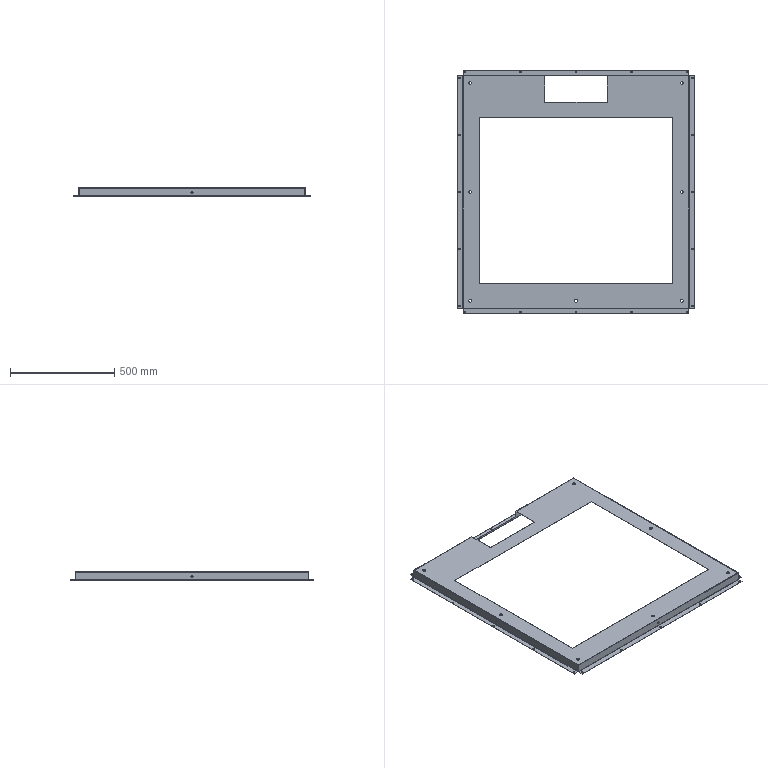Part | 1 solid | 194 faces | box 1139 x 1169 x 40 mm | volume 708675 mm3 | plane 98 | cylinder 88 | spline 8 | commonest cylinder face diameters 7 x50 14 x14 0.4 x9 2.4 x9 10 x6